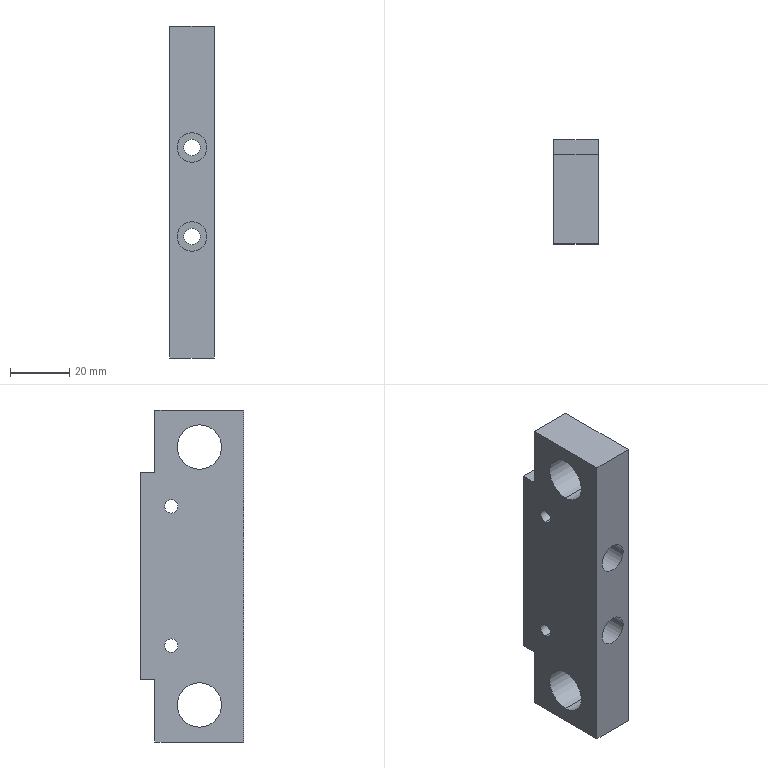Part | STEP file | 02-22 Push connecting block | 1 solid | 34 faces | box 15 x 35 x 112 mm | volume 46704 mm3 | cylinder 20 | plane 14 | commonest cylinder face diameters 4.5 x4 5.5 x4 8.5 x4 10 x4 15 x4